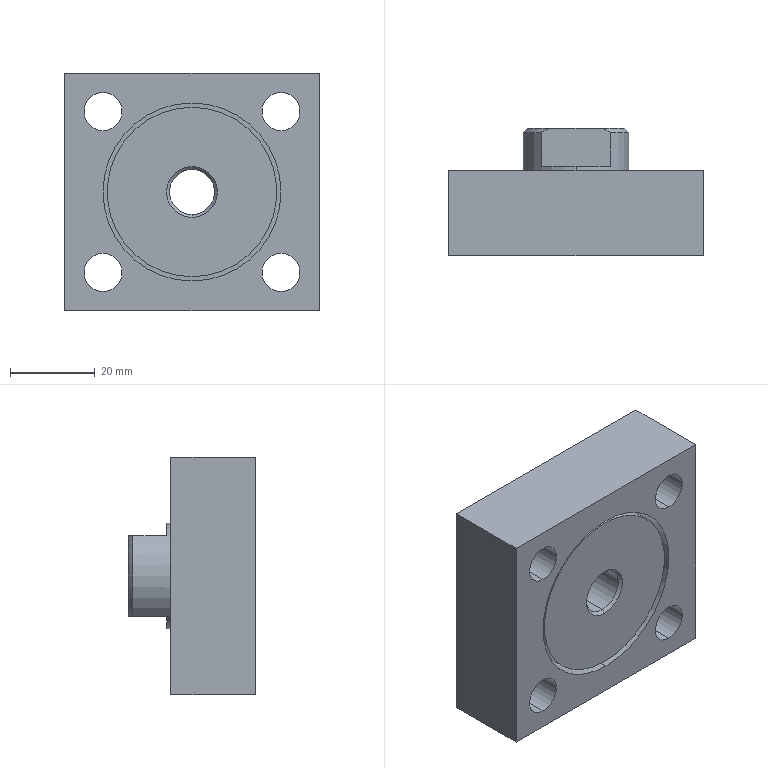Part | SolidWorks | features BaseBody 1 | 1 solid | 51 faces | box 60 x 30 x 56 mm | volume 57044 mm3 | cylinder 26 | plane 18 | cone 7 | commonest cylinder face diameters 9 x8 15 x8 10.647 x2 25 x2 27 x2 40 x2
STEP:
#1=CARTESIAN_POINT('',(21.,11.,11.5));
#2=VERTEX_POINT('',#1);
#3=CARTESIAN_POINT('',(21.,11.,26.5));
#4=VERTEX_POINT('',#3);
#5=CARTESIAN_POINT('',(21.,11.,19.));
#6=DIRECTION('',(0.,1.,0.));
#7=DIRECTION('',(0.,0.,1.));
#8=AXIS2_PLACEMENT_3D('',#5,#6,#7);
#9=CIRCLE('',#8,7.5);
#10=EDGE_CURVE('',#2,#4,#9,.T.);
#11=ORIENTED_EDGE('',*,*,#10,.F.);
#12=CARTESIAN_POINT('',(21.,20.,11.5));
#13=VERTEX_POINT('',#12);
#14=CARTESIAN_POINT('',(21.,0.,11.5));
#15=DIRECTION('',(0.,1.,0.));
#16=VECTOR('',#15,1000.);
#17=LINE('',#14,#16);
#18=EDGE_CURVE('',#2,#13,#17,.T.);
#19=ORIENTED_EDGE('',*,*,#18,.T.);
#20=CARTESIAN_POINT('',(21.,20.,26.5));
#21=VERTEX_POINT('',#20);
#22=CARTESIAN_POINT('',(21.,20.,19.));
#23=DIRECTION('',(0.,-1.,0.));
#24=DIRECTION('',(0.,0.,1.));
#25=AXIS2_PLACEMENT_3D('',#22,#23,#24);
#26=CIRCLE('',#25,7.5);
#27=EDGE_CURVE('',#21,#13,#26,.T.);
#28=ORIENTED_EDGE('',*,*,#27,.F.);
#29=CARTESIAN_POINT('',(21.,0.,26.5));
#30=DIRECTION('',(0.,1.,0.));
#31=VECTOR('',#30,1000.);
#32=LINE('',#29,#31);
#33=EDGE_CURVE('',#4,#21,#32,.T.);
#34=ORIENTED_EDGE('',*,*,#33,.F.);
#35=EDGE_LOOP('',(#11,#19,#28,#34));
#36=FACE_OUTER_BOUND('',#35,.T.);
#37=CARTESIAN_POINT('',(21.,0.,19.));
#38=DIRECTION('',(0.,1.,0.));
#39=DIRECTION('',(0.,0.,1.));
#40=AXIS2_PLACEMENT_3D('',#37,#38,#39);
#41=CYLINDRICAL_SURFACE('',#40,7.5);
#42=ADVANCED_FACE('',(#36),#41,.F.);
#43=CARTESIAN_POINT('',(-21.,11.,11.5));
#44=VERTEX_POINT('',#43);
#45=CARTESIAN_POINT('',(-21.,11.,26.5));
#46=VERTEX_POINT('',#45);
#47=CARTESIAN_POINT('',(-21.,11.,19.));
#48=DIRECTION('',(0.,1.,0.));
#49=DIRECTION('',(0.,0.,1.));
#50=AXIS2_PLACEMENT_3D('',#47,#48,#49);
#51=CIRCLE('',#50,7.5);
#52=EDGE_CURVE('',#44,#46,#51,.T.);
#53=ORIENTED_EDGE('',*,*,#52,.F.);
#54=CARTESIAN_POINT('',(-21.,20.,11.5));
#55=VERTEX_POINT('',#54);
#56=CARTESIAN_POINT('',(-21.,0.,11.5));
#57=DIRECTION('',(0.,1.,0.));
#58=VECTOR('',#57,1000.);
#59=LINE('',#56,#58);
#60=EDGE_CURVE('',#44,#55,#59,.T.);
#61=ORIENTED_EDGE('',*,*,#60,.T.);
#62=CARTESIAN_POINT('',(-21.,20.,26.5));
#63=VERTEX_POINT('',#62);
#64=CARTESIAN_POINT('',(-21.,20.,19.));
#65=DIRECTION('',(0.,-1.,0.));
#66=DIRECTION('',(0.,0.,1.));
#67=AXIS2_PLACEMENT_3D('',#64,#65,#66);
#68=CIRCLE('',#67,7.5);
#69=EDGE_CURVE('',#63,#55,#68,.T.);
#70=ORIENTED_EDGE('',*,*,#69,.F.);
#71=CARTESIAN_POINT('',(-21.,0.,26.5));
#72=DIRECTION('',(0.,1.,0.));
#73=VECTOR('',#72,1000.);
#74=LINE('',#71,#73);
#75=EDGE_CURVE('',#46,#63,#74,.T.);
#76=ORIENTED_EDGE('',*,*,#75,.F.);
#77=EDGE_LOOP('',(#53,#61,#70,#76));
#78=FACE_OUTER_BOUND('',#77,.T.);
#79=CARTESIAN_POINT('',(-21.,0.,19.));
#80=DIRECTION('',(0.,1.,0.));
#81=DIRECTION('',(0.,0.,1.));
#82=AXIS2_PLACEMENT_3D('',#79,#80,#81);
#83=CYLINDRICAL_SURFACE('',#82,7.5);
#84=ADVANCED_FACE('',(#78),#83,.F.);
#85=CARTESIAN_POINT('',(-21.,11.,-26.5));
#86=VERTEX_POINT('',#85);
#87=CARTESIAN_POINT('',(-21.,11.,-11.5));
#88=VERTEX_POINT('',#87);
#89=CARTESIAN_POINT('',(-21.,11.,-19.));
#90=DIRECTION('',(0.,1.,0.));
#91=DIRECTION('',(0.,0.,1.));
#92=AXIS2_PLACEMENT_3D('',#89,#90,#91);
#93=CIRCLE('',#92,7.5);
#94=EDGE_CURVE('',#86,#88,#93,.T.);
#95=ORIENTED_EDGE('',*,*,#94,.F.);
#96=CARTESIAN_POINT('',(-21.,20.,-26.5));
#97=VERTEX_POINT('',#96);
#98=CARTESIAN_POINT('',(-21.,0.,-26.5));
#99=DIRECTION('',(0.,1.,0.));
#100=VECTOR('',#99,1000.);
#101=LINE('',#98,#100);
#102=EDGE_CURVE('',#86,#97,#101,.T.);
#103=ORIENTED_EDGE('',*,*,#102,.T.);
#104=CARTESIAN_POINT('',(-21.,20.,-11.5));
#105=VERTEX_POINT('',#104);
#106=CARTESIAN_POINT('',(-21.,20.,-19.));
#107=DIRECTION('',(0.,-1.,0.));
#108=DIRECTION('',(0.,0.,1.));
#109=AXIS2_PLACEMENT_3D('',#106,#107,#108);
#110=CIRCLE('',#109,7.5);
#111=EDGE_CURVE('',#105,#97,#110,.T.);
#112=ORIENTED_EDGE('',*,*,#111,.F.);
#113=CARTESIAN_POINT('',(-21.,0.,-11.5));
#114=DIRECTION('',(0.,1.,0.));
#115=VECTOR('',#114,1000.);
#116=LINE('',#113,#115);
#117=EDGE_CURVE('',#88,#105,#116,.T.);
#118=ORIENTED_EDGE('',*,*,#117,.F.);
#119=EDGE_LOOP('',(#95,#103,#112,#118));
#120=FACE_OUTER_BOUND('',#119,.T.);
#121=CARTESIAN_POINT('',(-21.,0.,-19.));
#122=DIRECTION('',(0.,1.,0.));
#123=DIRECTION('',(0.,0.,1.));
#124=AXIS2_PLACEMENT_3D('',#121,#122,#123);
#125=CYLINDRICAL_SURFACE('',#124,7.5);
#126=ADVANCED_FACE('',(#120),#125,.F.);
#127=CARTESIAN_POINT('',(21.,11.,-26.5));
#128=VERTEX_POINT('',#127);
#129=CARTESIAN_POINT('',(21.,11.,-11.5));
#130=VERTEX_POINT('',#129);
#131=CARTESIAN_POINT('',(21.,11.,-19.));
#132=DIRECTION('',(0.,1.,0.));
#133=DIRECTION('',(0.,0.,1.));
#134=AXIS2_PLACEMENT_3D('',#131,#132,#133);
#135=CIRCLE('',#134,7.5);
#136=EDGE_CURVE('',#128,#130,#135,.T.);
#137=ORIENTED_EDGE('',*,*,#136,.F.);
#138=CARTESIAN_POINT('',(21.,20.,-26.5));
#139=VERTEX_POINT('',#138);
#140=CARTESIAN_POINT('',(21.,0.,-26.5));
#141=DIRECTION('',(0.,1.,0.));
#142=VECTOR('',#141,1000.);
#143=LINE('',#140,#142);
#144=EDGE_CURVE('',#128,#139,#143,.T.);
#145=ORIENTED_EDGE('',*,*,#144,.T.);
#146=CARTESIAN_POINT('',(21.,20.,-11.5));
#147=VERTEX_POINT('',#146);
#148=CARTESIAN_POINT('',(21.,20.,-19.));
#149=DIRECTION('',(0.,-1.,0.));
#150=DIRECTION('',(0.,0.,1.));
#151=AXIS2_PLACEMENT_3D('',#148,#149,#150);
#152=CIRCLE('',#151,7.5);
#153=EDGE_CURVE('',#147,#139,#152,.T.);
#154=ORIENTED_EDGE('',*,*,#153,.F.);
#155=CARTESIAN_POINT('',(21.,0.,-11.5));
#156=DIRECTION('',(0.,1.,0.));
#157=VECTOR('',#156,1000.);
#158=LINE('',#155,#157);
#159=EDGE_CURVE('',#130,#147,#158,.T.);
#160=ORIENTED_EDGE('',*,*,#159,.F.);
#161=EDGE_LOOP('',(#137,#145,#154,#160));
#162=FACE_OUTER_BOUND('',#161,.T.);
#163=CARTESIAN_POINT('',(21.,0.,-19.));
#164=DIRECTION('',(0.,1.,0.));
#165=DIRECTION('',(0.,0.,1.));
#166=AXIS2_PLACEMENT_3D('',#163,#164,#165);
#167=CYLINDRICAL_SURFACE('',#166,7.5);
#168=ADVANCED_FACE('',(#162),#167,.F.);
#169=CARTESIAN_POINT('',(0.,8.,-13.5));
#170=VERTEX_POINT('',#169);
#171=CARTESIAN_POINT('',(0.,8.,13.5));
#172=VERTEX_POINT('',#171);
#173=CARTESIAN_POINT('',(0.,8.,0.));
#174=DIRECTION('',(0.,1.,0.));
#175=DIRECTION('',(0.,0.,1.));
#176=AXIS2_PLACEMENT_3D('',#173,#174,#175);
#177=CIRCLE('',#176,13.5);
#178=EDGE_CURVE('',#170,#172,#177,.T.);
#179=ORIENTED_EDGE('',*,*,#178,.F.);
#180=CARTESIAN_POINT('',(0.,20.,-13.5));
#181=VERTEX_POINT('',#180);
#182=CARTESIAN_POINT('',(0.,0.,-13.5));
#183=DIRECTION('',(0.,1.,0.));
#184=VECTOR('',#183,1000.);
#185=LINE('',#182,#184);
#186=EDGE_CURVE('',#170,#181,#185,.T.);
#187=ORIENTED_EDGE('',*,*,#186,.T.);
#188=CARTESIAN_POINT('',(0.,20.,13.5));
#189=VERTEX_POINT('',#188);
#190=CARTESIAN_POINT('',(0.,20.,0.));
#191=DIRECTION('',(0.,-1.,0.));
#192=DIRECTION('',(0.,0.,1.));
#193=AXIS2_PLACEMENT_3D('',#190,#191,#192);
#194=CIRCLE('',#193,13.5);
#195=EDGE_CURVE('',#189,#181,#194,.T.);
#196=ORIENTED_EDGE('',*,*,#195,.F.);
#197=CARTESIAN_POINT('',(0.,0.,13.5));
#198=DIRECTION('',(0.,1.,0.));
#199=VECTOR('',#198,1000.);
#200=LINE('',#197,#199);
#201=EDGE_CURVE('',#172,#189,#200,.T.);
#202=ORIENTED_EDGE('',*,*,#201,.F.);
#203=EDGE_LOOP('',(#179,#187,#196,#202));
#204=FACE_OUTER_BOUND('',#203,.T.);
#205=CARTESIAN_POINT('',(0.,0.,0.));
#206=DIRECTION('',(0.,1.,0.));
#207=DIRECTION('',(0.,0.,1.));
#208=AXIS2_PLACEMENT_3D('',#205,#206,#207);
#209=CYLINDRICAL_SURFACE('',#208,13.5);
#210=ADVANCED_FACE('',(#204),#209,.F.);
#211=CARTESIAN_POINT('',(21.,0.,23.5));
#212=VERTEX_POINT('',#211);
#213=CARTESIAN_POINT('',(21.,0.,14.5));
#214=VERTEX_POINT('',#213);
#215=CARTESIAN_POINT('',(21.,0.,19.));
#216=DIRECTION('',(0.,-1.,0.));
#217=DIRECTION('',(0.,0.,1.));
#218=AXIS2_PLACEMENT_3D('',#215,#216,#217);
#219=CIRCLE('',#218,4.5);
#220=EDGE_CURVE('',#212,#214,#219,.T.);
#221=ORIENTED_EDGE('',*,*,#220,.T.);
#222=CARTESIAN_POINT('',(21.,11.,14.5));
#223=VERTEX_POINT('',#222);
#224=CARTESIAN_POINT('',(21.,0.,14.5));
#225=DIRECTION('',(0.,1.,0.));
#226=VECTOR('',#225,1000.);
#227=LINE('',#224,#226);
#228=EDGE_CURVE('',#214,#223,#227,.T.);
#229=ORIENTED_EDGE('',*,*,#228,.T.);
#230=CARTESIAN_POINT('',(21.,11.,23.5));
#231=VERTEX_POINT('',#230);
#232=CARTESIAN_POINT('',(21.,11.,19.));
#233=DIRECTION('',(0.,-1.,0.));
#234=DIRECTION('',(0.,0.,1.));
#235=AXIS2_PLACEMENT_3D('',#232,#233,#234);
#236=CIRCLE('',#235,4.5);
#237=EDGE_CURVE('',#231,#223,#236,.T.);
#238=ORIENTED_EDGE('',*,*,#237,.F.);
#239=CARTESIAN_POINT('',(21.,0.,23.5));
#240=DIRECTION('',(0.,1.,0.));
#241=VECTOR('',#240,1000.);
#242=LINE('',#239,#241);
#243=EDGE_CURVE('',#212,#231,#242,.T.);
#244=ORIENTED_EDGE('',*,*,#243,.F.);
#245=EDGE_LOOP('',(#221,#229,#238,#244));
#246=FACE_OUTER_BOUND('',#245,.T.);
#247=CARTESIAN_POINT('',(21.,0.,19.));
#248=DIRECTION('',(0.,1.,0.));
#249=DIRECTION('',(0.,0.,1.));
#250=AXIS2_PLACEMENT_3D('',#247,#248,#249);
#251=CYLINDRICAL_SURFACE('',#250,4.5);
#252=ADVANCED_FACE('',(#246),#251,.F.);
#253=CARTESIAN_POINT('',(-21.,0.,23.5));
#254=VERTEX_POINT('',#253);
#255=CARTESIAN_POINT('',(-21.,0.,14.5));
#256=VERTEX_POINT('',#255);
#257=CARTESIAN_POINT('',(-21.,0.,19.));
#258=DIRECTION('',(0.,-1.,0.));
#259=DIRECTION('',(0.,0.,1.));
#260=AXIS2_PLACEMENT_3D('',#257,#258,#259);
#261=CIRCLE('',#260,4.5);
#262=EDGE_CURVE('',#254,#256,#261,.T.);
#263=ORIENTED_EDGE('',*,*,#262,.T.);
#264=CARTESIAN_POINT('',(-21.,11.,14.5));
#265=VERTEX_POINT('',#264);
#266=CARTESIAN_POINT('',(-21.,0.,14.5));
#267=DIRECTION('',(0.,1.,0.));
#268=VECTOR('',#267,1000.);
#269=LINE('',#266,#268);
#270=EDGE_CURVE('',#256,#265,#269,.T.);
#271=ORIENTED_EDGE('',*,*,#270,.T.);
#272=CARTESIAN_POINT('',(-21.,11.,23.5));
#273=VERTEX_POINT('',#272);
#274=CARTESIAN_POINT('',(-21.,11.,19.));
#275=DIRECTION('',(0.,-1.,0.));
#276=DIRECTION('',(0.,0.,1.));
#277=AXIS2_PLACEMENT_3D('',#274,#275,#276);
#278=CIRCLE('',#277,4.5);
#279=EDGE_CURVE('',#273,#265,#278,.T.);
#280=ORIENTED_EDGE('',*,*,#279,.F.);
#281=CARTESIAN_POINT('',(-21.,0.,23.5));
#282=DIRECTION('',(0.,1.,0.));
#283=VECTOR('',#282,1000.);
#284=LINE('',#281,#283);
#285=EDGE_CURVE('',#254,#273,#284,.T.);
#286=ORIENTED_EDGE('',*,*,#285,.F.);
#287=EDGE_LOOP('',(#263,#271,#280,#286));
#288=FACE_OUTER_BOUND('',#287,.T.);
#289=CARTESIAN_POINT('',(-21.,0.,19.));
#290=DIRECTION('',(0.,1.,0.));
#291=DIRECTION('',(0.,0.,1.));
#292=AXIS2_PLACEMENT_3D('',#289,#290,#291);
#293=CYLINDRICAL_SURFACE('',#292,4.5);
#294=ADVANCED_FACE('',(#288),#293,.F.);
#295=CARTESIAN_POINT('',(-21.,0.,-14.5));
#296=VERTEX_POINT('',#295);
#297=CARTESIAN_POINT('',(-21.,0.,-23.5));
#298=VERTEX_POINT('',#297);
#299=CARTESIAN_POINT('',(-21.,0.,-19.));
#300=DIRECTION('',(0.,-1.,0.));
#301=DIRECTION('',(0.,0.,1.));
#302=AXIS2_PLACEMENT_3D('',#299,#300,#301);
#303=CIRCLE('',#302,4.5);
#304=EDGE_CURVE('',#296,#298,#303,.T.);
#305=ORIENTED_EDGE('',*,*,#304,.T.);
#306=CARTESIAN_POINT('',(-21.,11.,-23.5));
#307=VERTEX_POINT('',#306);
#308=CARTESIAN_POINT('',(-21.,0.,-23.5));
#309=DIRECTION('',(0.,1.,0.));
#310=VECTOR('',#309,1000.);
#311=LINE('',#308,#310);
#312=EDGE_CURVE('',#298,#307,#311,.T.);
#313=ORIENTED_EDGE('',*,*,#312,.T.);
#314=CARTESIAN_POINT('',(-21.,11.,-14.5));
#315=VERTEX_POINT('',#314);
#316=CARTESIAN_POINT('',(-21.,11.,-19.));
#317=DIRECTION('',(0.,-1.,0.));
#318=DIRECTION('',(0.,0.,1.));
#319=AXIS2_PLACEMENT_3D('',#316,#317,#318);
#320=CIRCLE('',#319,4.5);
#321=EDGE_CURVE('',#315,#307,#320,.T.);
#322=ORIENTED_EDGE('',*,*,#321,.F.);
#323=CARTESIAN_POINT('',(-21.,0.,-14.5));
#324=DIRECTION('',(0.,1.,0.));
#325=VECTOR('',#324,1000.);
#326=LINE('',#323,#325);
#327=EDGE_CURVE('',#296,#315,#326,.T.);
#328=ORIENTED_EDGE('',*,*,#327,.F.);
#329=EDGE_LOOP('',(#305,#313,#322,#328));
#330=FACE_OUTER_BOUND('',#329,.T.);
#331=CARTESIAN_POINT('',(-21.,0.,-19.));
#332=DIRECTION('',(0.,1.,0.));
#333=DIRECTION('',(0.,0.,1.));
#334=AXIS2_PLACEMENT_3D('',#331,#332,#333);
#335=CYLINDRICAL_SURFACE('',#334,4.5);
#336=ADVANCED_FACE('',(#330),#335,.F.);
#337=CARTESIAN_POINT('',(21.,0.,-14.5));
#338=VERTEX_POINT('',#337);
#339=CARTESIAN_POINT('',(21.,0.,-23.5));
#340=VERTEX_POINT('',#339);
#341=CARTESIAN_POINT('',(21.,0.,-19.));
#342=DIRECTION('',(0.,-1.,0.));
#343=DIRECTION('',(0.,0.,1.));
#344=AXIS2_PLACEMENT_3D('',#341,#342,#343);
#345=CIRCLE('',#344,4.5);
#346=EDGE_CURVE('',#338,#340,#345,.T.);
#347=ORIENTED_EDGE('',*,*,#346,.T.);
#348=CARTESIAN_POINT('',(21.,11.,-23.5));
#349=VERTEX_POINT('',#348);
#350=CARTESIAN_POINT('',(21.,0.,-23.5));
#351=DIRECTION('',(0.,1.,0.));
#352=VECTOR('',#351,1000.);
#353=LINE('',#350,#352);
#354=EDGE_CURVE('',#340,#349,#353,.T.);
#355=ORIENTED_EDGE('',*,*,#354,.T.);
#356=CARTESIAN_POINT('',(21.,11.,-14.5));
#357=VERTEX_POINT('',#356);
#358=CARTESIAN_POINT('',(21.,11.,-19.));
#359=DIRECTION('',(0.,-1.,0.));
#360=DIRECTION('',(0.,0.,1.));
#361=AXIS2_PLACEMENT_3D('',#358,#359,#360);
#362=CIRCLE('',#361,4.5);
#363=EDGE_CURVE('',#357,#349,#362,.T.);
#364=ORIENTED_EDGE('',*,*,#363,.F.);
#365=CARTESIAN_POINT('',(21.,0.,-14.5));
#366=DIRECTION('',(0.,1.,0.));
#367=VECTOR('',#366,1000.);
#368=LINE('',#365,#367);
#369=EDGE_CURVE('',#338,#357,#368,.T.);
#370=ORIENTED_EDGE('',*,*,#369,.F.);
#371=EDGE_LOOP('',(#347,#355,#364,#370));
#372=FACE_OUTER_BOUND('',#371,.T.);
#373=CARTESIAN_POINT('',(21.,0.,-19.));
#374=DIRECTION('',(0.,1.,0.));
#375=DIRECTION('',(0.,0.,1.));
#376=AXIS2_PLACEMENT_3D('',#373,#374,#375);
#377=CYLINDRICAL_SURFACE('',#376,4.5);
#378=ADVANCED_FACE('',(#372),#377,.F.);
#379=CARTESIAN_POINT('',(0.,0.,21.));
#380=VERTEX_POINT('',#379);
#381=CARTESIAN_POINT('',(0.,0.,-21.));
#382=VERTEX_POINT('',#381);
#383=CARTESIAN_POINT('',(0.,0.,0.));
#384=DIRECTION('',(0.,-1.,0.));
#385=DIRECTION('',(0.,0.,1.));
#386=AXIS2_PLACEMENT_3D('',#383,#384,#385);
#387=CIRCLE('',#386,21.);
#388=EDGE_CURVE('',#380,#382,#387,.T.);
#389=ORIENTED_EDGE('',*,*,#388,.T.);
#390=CARTESIAN_POINT('',(0.,8.,-21.));
#391=VERTEX_POINT('',#390);
#392=CARTESIAN_POINT('',(0.,0.,-21.));
#393=DIRECTION('',(0.,1.,0.));
#394=VECTOR('',#393,1000.);
#395=LINE('',#392,#394);
#396=EDGE_CURVE('',#382,#391,#395,.T.);
#397=ORIENTED_EDGE('',*,*,#396,.T.);
#398=CARTESIAN_POINT('',(0.,8.,21.));
#399=VERTEX_POINT('',#398);
#400=CARTESIAN_POINT('',(0.,8.,0.));
#401=DIRECTION('',(0.,-1.,0.));
#402=DIRECTION('',(0.,0.,1.));
#403=AXIS2_PLACEMENT_3D('',#400,#401,#402);
#404=CIRCLE('',#403,21.);
#405=EDGE_CURVE('',#399,#391,#404,.T.);
#406=ORIENTED_EDGE('',*,*,#405,.F.);
#407=CARTESIAN_POINT('',(0.,0.,21.));
#408=DIRECTION('',(0.,1.,0.));
#409=VECTOR('',#408,1000.);
#410=LINE('',#407,#409);
#411=EDGE_CURVE('',#380,#399,#410,.T.);
#412=ORIENTED_EDGE('',*,*,#411,.F.);
#413=EDGE_LOOP('',(#389,#397,#406,#412));
#414=FACE_OUTER_BOUND('',#413,.T.);
#415=CARTESIAN_POINT('',(0.,0.,0.));
#416=DIRECTION('',(0.,1.,0.));
#417=DIRECTION('',(0.,0.,1.));
#418=AXIS2_PLACEMENT_3D('',#415,#416,#417);
#419=CYLINDRICAL_SURFACE('',#418,21.);
#420=ADVANCED_FACE('',(#414),#419,.F.);
#421=CARTESIAN_POINT('',(0.,8.,-12.5));
#422=VERTEX_POINT('',#421);
#423=CARTESIAN_POINT('',(0.,8.,12.5));
#424=VERTEX_POINT('',#423);
#425=CARTESIAN_POINT('',(0.,8.,0.));
#426=DIRECTION('',(0.,-1.,0.));
#427=DIRECTION('',(0.,0.,1.));
#428=AXIS2_PLACEMENT_3D('',#425,#426,#427);
#429=CIRCLE('',#428,12.5);
#430=EDGE_CURVE('',#422,#424,#429,.T.);
#431=ORIENTED_EDGE('',*,*,#430,.F.);
#432=CARTESIAN_POINT('',(0.,21.,-12.5));
#433=VERTEX_POINT('',#432);
#434=CARTESIAN_POINT('',(0.,0.5,-12.5));
#435=DIRECTION('',(0.,1.,0.));
#436=VECTOR('',#435,1000.);
#437=LINE('',#434,#436);
#438=EDGE_CURVE('',#422,#433,#437,.T.);
#439=ORIENTED_EDGE('',*,*,#438,.T.);
#440=CARTESIAN_POINT('',(8.124,21.,-9.5));
#441=VERTEX_POINT('',#440);
#442=CARTESIAN_POINT('',(0.,21.,0.));
#443=DIRECTION('',(0.,-1.,0.));
#444=DIRECTION('',(0.,0.,1.));
#445=AXIS2_PLACEMENT_3D('',#442,#443,#444);
#446=CIRCLE('',#445,12.5);
#447=EDGE_CURVE('',#433,#441,#446,.T.);
#448=ORIENTED_EDGE('',*,*,#447,.T.);
#449=CARTESIAN_POINT('',(8.124,29.,-9.5));
#450=VERTEX_POINT('',#449);
#451=CARTESIAN_POINT('',(8.124,0.5,-9.5));
#452=DIRECTION('',(0.,1.,0.));
#453=VECTOR('',#452,1000.);
#454=LINE('',#451,#453);
#455=EDGE_CURVE('',#441,#450,#454,.T.);
#456=ORIENTED_EDGE('',*,*,#455,.T.);
#457=CARTESIAN_POINT('',(12.5,29.,0.));
#458=VERTEX_POINT('',#457);
#459=CARTESIAN_POINT('',(0.,29.,0.));
#460=DIRECTION('',(0.,-1.,0.));
#461=DIRECTION('',(0.,0.,1.));
#462=AXIS2_PLACEMENT_3D('',#459,#460,#461);
#463=CIRCLE('',#462,12.5);
#464=EDGE_CURVE('',#450,#458,#463,.T.);
#465=ORIENTED_EDGE('',*,*,#464,.T.);
#466=CARTESIAN_POINT('',(8.124,29.,9.5));
#467=VERTEX_POINT('',#466);
#468=CARTESIAN_POINT('',(0.,29.,0.));
#469=DIRECTION('',(0.,-1.,0.));
#470=DIRECTION('',(0.,0.,1.));
#471=AXIS2_PLACEMENT_3D('',#468,#469,#470);
#472=CIRCLE('',#471,12.5);
#473=EDGE_CURVE('',#458,#467,#472,.T.);
#474=ORIENTED_EDGE('',*,*,#473,.T.);
#475=CARTESIAN_POINT('',(8.124,21.,9.5));
#476=VERTEX_POINT('',#475);
#477=CARTESIAN_POINT('',(8.124,0.5,9.5));
#478=DIRECTION('',(0.,-1.,0.));
#479=VECTOR('',#478,1000.);
#480=LINE('',#477,#479);
#481=EDGE_CURVE('',#467,#476,#480,.T.);
#482=ORIENTED_EDGE('',*,*,#481,.T.);
#483=CARTESIAN_POINT('',(0.,21.,12.5));
#484=VERTEX_POINT('',#483);
#485=CARTESIAN_POINT('',(0.,21.,0.));
#486=DIRECTION('',(0.,-1.,0.));
#487=DIRECTION('',(0.,0.,1.));
#488=AXIS2_PLACEMENT_3D('',#485,#486,#487);
#489=CIRCLE('',#488,12.5);
#490=EDGE_CURVE('',#476,#484,#489,.T.);
#491=ORIENTED_EDGE('',*,*,#490,.T.);
#492=CARTESIAN_POINT('',(0.,0.5,12.5));
#493=DIRECTION('',(0.,1.,0.));
#494=VECTOR('',#493,1000.);
#495=LINE('',#492,#494);
#496=EDGE_CURVE('',#424,#484,#495,.T.);
#497=ORIENTED_EDGE('',*,*,#496,.F.);
#498=EDGE_LOOP('',(#431,#439,#448,#456,#465,#474,#482,#491,#497));
#499=FACE_OUTER_BOUND('',#498,.T.);
#500=CARTESIAN_POINT('',(0.,0.5,0.));
#501=DIRECTION('',(0.,1.,0.));
#502=DIRECTION('',(0.,0.,1.));
#503=AXIS2_PLACEMENT_3D('',#500,#501,#502);
#504=CYLINDRICAL_SURFACE('',#503,12.5);
#505=ADVANCED_FACE('',(#499),#504,.T.);
#506=CARTESIAN_POINT('',(6.481,30.,-9.5));
#507=VERTEX_POINT('',#506);
#508=CARTESIAN_POINT('',(11.5,30.,0.));
#509=VERTEX_POINT('',#508);
#510=CARTESIAN_POINT('',(0.,30.,0.));
#511=DIRECTION('',(0.,-1.,0.));
#512=DIRECTION('',(1.,0.,0.));
#513=AXIS2_PLACEMENT_3D('',#510,#511,#512);
#514=CIRCLE('',#513,11.5);
#515=EDGE_CURVE('',#507,#509,#514,.T.);
#516=ORIENTED_EDGE('',*,*,#515,.T.);
#517=CARTESIAN_POINT('',(12.5,29.,0.));
#518=DIRECTION('',(0.7071,-0.7071,0.));
#519=VECTOR('',#518,1000.);
#520=LINE('',#517,#519);
#521=EDGE_CURVE('',#509,#458,#520,.T.);
#522=ORIENTED_EDGE('',*,*,#521,.T.);
#523=ORIENTED_EDGE('',*,*,#464,.F.);
#524=CARTESIAN_POINT('',(8.124,29.,-9.5));
#525=CARTESIAN_POINT('',(7.586,29.35,-9.5));
#526=CARTESIAN_POINT('',(7.04,29.685,-9.5));
#527=CARTESIAN_POINT('',(6.481,30.,-9.5));
#528=B_SPLINE_CURVE_WITH_KNOTS('',3,(#524,#525,#526,#527),.UNSPECIFIED.,.F.,.F.,(4,4),(0.,0.001924),.UNSPECIFIED.);
#529=EDGE_CURVE('',#450,#507,#528,.T.);
#530=ORIENTED_EDGE('',*,*,#529,.T.);
#531=EDGE_LOOP('',(#516,#522,#523,#530));
#532=FACE_OUTER_BOUND('',#531,.T.);
#533=CARTESIAN_POINT('',(0.,29.,0.));
#534=DIRECTION('',(0.,-1.,0.));
#535=DIRECTION('',(1.,0.,0.));
#536=AXIS2_PLACEMENT_3D('',#533,#534,#535);
#537=CONICAL_SURFACE('',#536,12.5,0.7854);
#538=ADVANCED_FACE('',(#532),#537,.T.);
#539=CARTESIAN_POINT('',(0.,0.5,20.));
#540=VERTEX_POINT('',#539);
#541=CARTESIAN_POINT('',(0.,0.5,-20.));
#542=VERTEX_POINT('',#541);
#543=CARTESIAN_POINT('',(0.,0.5,0.));
#544=DIRECTION('',(0.,1.,0.));
#545=DIRECTION('',(0.,0.,1.));
#546=AXIS2_PLACEMENT_3D('',#543,#544,#545);
#547=CIRCLE('',#546,20.);
#548=EDGE_CURVE('',#540,#542,#547,.T.);
#549=ORIENTED_EDGE('',*,*,#548,.T.);
#550=CARTESIAN_POINT('',(0.,8.,-20.));
#551=VERTEX_POINT('',#550);
#552=CARTESIAN_POINT('',(0.,0.5,-20.));
#553=DIRECTION('',(0.,1.,0.));
#554=VECTOR('',#553,1000.);
#555=LINE('',#552,#554);
#556=EDGE_CURVE('',#542,#551,#555,.T.);
#557=ORIENTED_EDGE('',*,*,#556,.T.);
#558=CARTESIAN_POINT('',(0.,8.,20.));
#559=VERTEX_POINT('',#558);
#560=CARTESIAN_POINT('',(0.,8.,0.));
#561=DIRECTION('',(0.,1.,0.));
#562=DIRECTION('',(0.,0.,1.));
#563=AXIS2_PLACEMENT_3D('',#560,#561,#562);
#564=CIRCLE('',#563,20.);
#565=EDGE_CURVE('',#559,#551,#564,.T.);
#566=ORIENTED_EDGE('',*,*,#565,.F.);
#567=CARTESIAN_POINT('',(0.,0.5,20.));
#568=DIRECTION('',(0.,1.,0.));
#569=VECTOR('',#568,1000.);
#570=LINE('',#567,#569);
#571=EDGE_CURVE('',#540,#559,#570,.T.);
#572=ORIENTED_EDGE('',*,*,#571,.F.);
#573=EDGE_LOOP('',(#549,#557,#566,#572));
#574=FACE_OUTER_BOUND('',#573,.T.);
#575=CARTESIAN_POINT('',(0.,0.5,0.));
#576=DIRECTION('',(0.,1.,0.));
#577=DIRECTION('',(0.,0.,1.));
#578=AXIS2_PLACEMENT_3D('',#575,#576,#577);
#579=CYLINDRICAL_SURFACE('',#578,20.);
#580=ADVANCED_FACE('',(#574),#579,.T.);
#581=CARTESIAN_POINT('',(0.,29.324,-5.323));
#582=VERTEX_POINT('',#581);
#583=CARTESIAN_POINT('',(0.,29.324,5.323));
#584=VERTEX_POINT('',#583);
#585=CARTESIAN_POINT('',(0.,29.324,0.));
#586=DIRECTION('',(0.,1.,0.));
#587=DIRECTION('',(0.,0.,1.));
#588=AXIS2_PLACEMENT_3D('',#585,#586,#587);
#589=CIRCLE('',#588,5.323);
#590=EDGE_CURVE('',#582,#584,#589,.T.);
#591=ORIENTED_EDGE('',*,*,#590,.F.);
#592=CARTESIAN_POINT('',(0.,30.,-6.));
#593=VERTEX_POINT('',#592);
#594=CARTESIAN_POINT('',(0.,30.,-6.));
#595=DIRECTION('',(0.,0.7071,-0.7071));
#596=VECTOR('',#595,1000.);
#597=LINE('',#594,#596);
#598=EDGE_CURVE('',#582,#593,#597,.T.);
#599=ORIENTED_EDGE('',*,*,#598,.T.);
#600=CARTESIAN_POINT('',(0.,30.,6.));
#601=VERTEX_POINT('',#600);
#602=CARTESIAN_POINT('',(0.,30.,0.));
#603=DIRECTION('',(0.,-1.,0.));
#604=DIRECTION('',(0.,0.,1.));
#605=AXIS2_PLACEMENT_3D('',#602,#603,#604);
#606=CIRCLE('',#605,6.);
#607=EDGE_CURVE('',#601,#593,#606,.T.);
#608=ORIENTED_EDGE('',*,*,#607,.F.);
#609=CARTESIAN_POINT('',(0.,30.,6.));
#610=DIRECTION('',(0.,0.7071,0.7071));
#611=VECTOR('',#610,1000.);
#612=LINE('',#609,#611);
#613=EDGE_CURVE('',#584,#601,#612,.T.);
#614=ORIENTED_EDGE('',*,*,#613,.F.);
#615=EDGE_LOOP('',(#591,#599,#608,#614));
#616=FACE_OUTER_BOUND('',#615,.T.);
#617=CARTESIAN_POINT('',(0.,30.,0.));
#618=DIRECTION('',(0.,1.,0.));
#619=DIRECTION('',(0.,0.,1.));
#620=AXIS2_PLACEMENT_3D('',#617,#618,#619);
#621=CONICAL_SURFACE('',#620,6.,0.7854);
#622=ADVANCED_FACE('',(#616),#621,.F.);
#623=CARTESIAN_POINT('',(0.,1.176,5.324));
#624=VERTEX_POINT('',#623);
#625=CARTESIAN_POINT('',(0.,1.176,-5.324));
#626=VERTEX_POINT('',#625);
#627=CARTESIAN_POINT('',(0.,1.176,0.));
#628=DIRECTION('',(0.,-1.,0.));
#629=DIRECTION('',(0.,0.,-1.));
#630=AXIS2_PLACEMENT_3D('',#627,#628,#629);
#631=CIRCLE('',#630,5.324);
#632=EDGE_CURVE('',#624,#626,#631,.T.);
#633=ORIENTED_EDGE('',*,*,#632,.F.);
#634=CARTESIAN_POINT('',(0.,0.5,6.));
#635=VERTEX_POINT('',#634);
#636=CARTESIAN_POINT('',(0.,0.5,6.));
#637=DIRECTION('',(0.,-0.7071,0.7071));
#638=VECTOR('',#637,1000.);
#639=LINE('',#636,#638);
#640=EDGE_CURVE('',#624,#635,#639,.T.);
#641=ORIENTED_EDGE('',*,*,#640,.T.);
#642=CARTESIAN_POINT('',(0.,0.5,-6.));
#643=VERTEX_POINT('',#642);
#644=CARTESIAN_POINT('',(0.,0.5,0.));
#645=DIRECTION('',(0.,1.,0.));
#646=DIRECTION('',(0.,0.,-1.));
#647=AXIS2_PLACEMENT_3D('',#644,#645,#646);
#648=CIRCLE('',#647,6.);
#649=EDGE_CURVE('',#643,#635,#648,.T.);
#650=ORIENTED_EDGE('',*,*,#649,.F.);
#651=CARTESIAN_POINT('',(0.,0.5,-6.));
#652=DIRECTION('',(0.,-0.7071,-0.7071));
#653=VECTOR('',#652,1000.);
#654=LINE('',#651,#653);
#655=EDGE_CURVE('',#626,#643,#654,.T.);
#656=ORIENTED_EDGE('',*,*,#655,.F.);
#657=EDGE_LOOP('',(#633,#641,#650,#656));
#658=FACE_OUTER_BOUND('',#657,.T.);
#659=CARTESIAN_POINT('',(0.,0.5,0.));
#660=DIRECTION('',(0.,-1.,0.));
#661=DIRECTION('',(0.,0.,-1.));
#662=AXIS2_PLACEMENT_3D('',#659,#660,#661);
#663=CONICAL_SURFACE('',#662,6.,0.7854);
#664=ADVANCED_FACE('',(#658),#663,.F.);
#665=ORIENTED_EDGE('',*,*,#632,.T.);
#666=CARTESIAN_POINT('',(0.,0.5,-5.324));
#667=DIRECTION('',(0.,1.,0.));
#668=VECTOR('',#667,1000.);
#669=LINE('',#666,#668);
#670=EDGE_CURVE('',#626,#582,#669,.T.);
#671=ORIENTED_EDGE('',*,*,#670,.T.);
#672=ORIENTED_EDGE('',*,*,#590,.T.);
#673=CARTESIAN_POINT('',(0.,0.5,5.324));
#674=DIRECTION('',(0.,1.,0.));
#675=VECTOR('',#674,1000.);
#676=LINE('',#673,#675);
#677=EDGE_CURVE('',#624,#584,#676,.T.);
#678=ORIENTED_EDGE('',*,*,#677,.F.);
#679=EDGE_LOOP('',(#665,#671,#672,#678));
#680=FACE_OUTER_BOUND('',#679,.T.);
#681=CARTESIAN_POINT('',(0.,0.5,0.));
#682=DIRECTION('',(0.,1.,0.));
#683=DIRECTION('',(0.,0.,1.));
#684=AXIS2_PLACEMENT_3D('',#681,#682,#683);
#685=CYLINDRICAL_SURFACE('',#684,5.324);
#686=ADVANCED_FACE('',(#680),#685,.F.);
#687=CARTESIAN_POINT('',(30.,20.,28.));
#688=VERTEX_POINT('',#687);
#689=CARTESIAN_POINT('',(30.,20.,-28.));
#690=VERTEX_POINT('',#689);
#691=CARTESIAN_POINT('',(30.,20.,0.));
#692=DIRECTION('',(0.,0.,-1.));
#693=VECTOR('',#692,1000.);
#694=LINE('',#691,#693);
#695=EDGE_CURVE('',#688,#690,#694,.T.);
#696=ORIENTED_EDGE('',*,*,#695,.T.);
#697=CARTESIAN_POINT('',(-30.,20.,-28.));
#698=VERTEX_POINT('',#697);
#699=CARTESIAN_POINT('',(0.,20.,-28.));
#700=DIRECTION('',(-1.,0.,0.));
#701=VECTOR('',#700,1000.);
#702=LINE('',#699,#701);
#703=EDGE_CURVE('',#690,#698,#702,.T.);
#704=ORIENTED_EDGE('',*,*,#703,.T.);
#705=CARTESIAN_POINT('',(-30.,20.,28.));
#706=VERTEX_POINT('',#705);
#707=CARTESIAN_POINT('',(-30.,20.,0.));
#708=DIRECTION('',(0.,0.,1.));
#709=VECTOR('',#708,1000.);
#710=LINE('',#707,#709);
#711=EDGE_CURVE('',#698,#706,#710,.T.);
#712=ORIENTED_EDGE('',*,*,#711,.T.);
#713=CARTESIAN_POINT('',(0.,20.,28.));
#714=DIRECTION('',(1.,0.,0.));
#715=VECTOR('',#714,1000.);
#716=LINE('',#713,#715);
#717=EDGE_CURVE('',#706,#688,#716,.T.);
#718=ORIENTED_EDGE('',*,*,#717,.T.);
#719=EDGE_LOOP('',(#696,#704,#712,#718));
#720=FACE_OUTER_BOUND('',#719,.T.);
#721=ORIENTED_EDGE('',*,*,#27,.T.);
#722=CARTESIAN_POINT('',(21.,20.,19.));
#723=DIRECTION('',(0.,-1.,0.));
#724=DIRECTION('',(0.,0.,1.));
#725=AXIS2_PLACEMENT_3D('',#722,#723,#724);
#726=CIRCLE('',#725,7.5);
#727=EDGE_CURVE('',#13,#21,#726,.T.);
#728=ORIENTED_EDGE('',*,*,#727,.T.);
#729=EDGE_LOOP('',(#721,#728));
#730=FACE_BOUND('',#729,.T.);
#731=ORIENTED_EDGE('',*,*,#69,.T.);
#732=CARTESIAN_POINT('',(-21.,20.,19.));
#733=DIRECTION('',(0.,-1.,0.));
#734=DIRECTION('',(0.,0.,1.));
#735=AXIS2_PLACEMENT_3D('',#732,#733,#734);
#736=CIRCLE('',#735,7.5);
#737=EDGE_CURVE('',#55,#63,#736,.T.);
#738=ORIENTED_EDGE('',*,*,#737,.T.);
#739=EDGE_LOOP('',(#731,#738));
#740=FACE_BOUND('',#739,.T.);
#741=ORIENTED_EDGE('',*,*,#111,.T.);
#742=CARTESIAN_POINT('',(-21.,20.,-19.));
#743=DIRECTION('',(0.,-1.,0.));
#744=DIRECTION('',(0.,0.,1.));
#745=AXIS2_PLACEMENT_3D('',#742,#743,#744);
#746=CIRCLE('',#745,7.5);
#747=EDGE_CURVE('',#97,#105,#746,.T.);
#748=ORIENTED_EDGE('',*,*,#747,.T.);
#749=EDGE_LOOP('',(#741,#748));
#750=FACE_BOUND('',#749,.T.);
#751=ORIENTED_EDGE('',*,*,#153,.T.);
#752=CARTESIAN_POINT('',(21.,20.,-19.));
#753=DIRECTION('',(0.,-1.,0.));
#754=DIRECTION('',(0.,0.,1.));
#755=AXIS2_PLACEMENT_3D('',#752,#753,#754);
#756=CIRCLE('',#755,7.5);
#757=EDGE_CURVE('',#139,#147,#756,.T.);
#758=ORIENTED_EDGE('',*,*,#757,.T.);
#759=EDGE_LOOP('',(#751,#758));
#760=FACE_BOUND('',#759,.T.);
#761=ORIENTED_EDGE('',*,*,#195,.T.);
#762=CARTESIAN_POINT('',(0.,20.,0.));
#763=DIRECTION('',(0.,-1.,0.));
#764=DIRECTION('',(0.,0.,1.));
#765=AXIS2_PLACEMENT_3D('',#762,#763,#764);
#766=CIRCLE('',#765,13.5);
#767=EDGE_CURVE('',#181,#189,#766,.T.);
#768=ORIENTED_EDGE('',*,*,#767,.T.);
#769=EDGE_LOOP('',(#761,#768));
#770=FACE_BOUND('',#769,.T.);
#771=CARTESIAN_POINT('',(0.,20.,0.));
#772=DIRECTION('',(0.,1.,0.));
#773=DIRECTION('',(0.,0.,1.));
#774=AXIS2_PLACEMENT_3D('',#771,#772,#773);
#775=PLANE('',#774);
#776=ADVANCED_FACE('',(#720,#730,#740,#750,#760,#770),#775,.T.);
#777=CARTESIAN_POINT('',(-30.,0.,-28.));
#778=VERTEX_POINT('',#777);
#779=CARTESIAN_POINT('',(-30.,20.,-28.));
#780=DIRECTION('',(0.,-1.,0.));
#781=VECTOR('',#780,1000.);
#782=LINE('',#779,#781);
#783=EDGE_CURVE('',#698,#778,#782,.T.);
#784=ORIENTED_EDGE('',*,*,#783,.F.);
#785=ORIENTED_EDGE('',*,*,#703,.F.);
#786=CARTESIAN_POINT('',(30.,0.,-28.));
#787=VERTEX_POINT('',#786);
#788=CARTESIAN_POINT('',(30.,20.,-28.));
#789=DIRECTION('',(0.,1.,0.));
#790=VECTOR('',#789,1000.);
#791=LINE('',#788,#790);
#792=EDGE_CURVE('',#787,#690,#791,.T.);
#793=ORIENTED_EDGE('',*,*,#792,.F.);
#794=CARTESIAN_POINT('',(30.,0.,-28.));
#795=DIRECTION('',(1.,0.,0.));
#796=VECTOR('',#795,1000.);
#797=LINE('',#794,#796);
#798=EDGE_CURVE('',#778,#787,#797,.T.);
#799=ORIENTED_EDGE('',*,*,#798,.F.);
#800=EDGE_LOOP('',(#784,#785,#793,#799));
#801=FACE_OUTER_BOUND('',#800,.T.);
#802=CARTESIAN_POINT('',(30.,20.,-28.));
#803=DIRECTION('',(0.,0.,1.));
#804=DIRECTION('',(1.,0.,0.));
#805=AXIS2_PLACEMENT_3D('',#802,#803,#804);
#806=PLANE('',#805);
#807=ADVANCED_FACE('',(#801),#806,.F.);
#808=ORIENTED_EDGE('',*,*,#792,.T.);
#809=ORIENTED_EDGE('',*,*,#695,.F.);
#810=CARTESIAN_POINT('',(30.,0.,28.));
#811=VERTEX_POINT('',#810);
#812=CARTESIAN_POINT('',(30.,20.,28.));
#813=DIRECTION('',(0.,1.,0.));
#814=VECTOR('',#813,1000.);
#815=LINE('',#812,#814);
#816=EDGE_CURVE('',#811,#688,#815,.T.);
#817=ORIENTED_EDGE('',*,*,#816,.F.);
#818=CARTESIAN_POINT('',(30.,0.,28.));
#819=DIRECTION('',(0.,0.,1.));
#820=VECTOR('',#819,1000.);
#821=LINE('',#818,#820);
#822=EDGE_CURVE('',#787,#811,#821,.T.);
#823=ORIENTED_EDGE('',*,*,#822,.F.);
#824=EDGE_LOOP('',(#808,#809,#817,#823));
#825=FACE_OUTER_BOUND('',#824,.T.);
#826=CARTESIAN_POINT('',(30.,20.,28.));
#827=DIRECTION('',(-1.,0.,0.));
#828=DIRECTION('',(0.,0.,1.));
#829=AXIS2_PLACEMENT_3D('',#826,#827,#828);
#830=PLANE('',#829);
#831=ADVANCED_FACE('',(#825),#830,.F.);
#832=ORIENTED_EDGE('',*,*,#816,.T.);
#833=ORIENTED_EDGE('',*,*,#717,.F.);
#834=CARTESIAN_POINT('',(-30.,0.,28.));
#835=VERTEX_POINT('',#834);
#836=CARTESIAN_POINT('',(-30.,20.,28.));
#837=DIRECTION('',(0.,1.,0.));
#838=VECTOR('',#837,1000.);
#839=LINE('',#836,#838);
#840=EDGE_CURVE('',#835,#706,#839,.T.);
#841=ORIENTED_EDGE('',*,*,#840,.F.);
#842=CARTESIAN_POINT('',(-30.,0.,28.));
#843=DIRECTION('',(-1.,0.,0.));
#844=VECTOR('',#843,1000.);
#845=LINE('',#842,#844);
#846=EDGE_CURVE('',#811,#835,#845,.T.);
#847=ORIENTED_EDGE('',*,*,#846,.F.);
#848=EDGE_LOOP('',(#832,#833,#841,#847));
#849=FACE_OUTER_BOUND('',#848,.T.);
#850=CARTESIAN_POINT('',(-30.,20.,28.));
#851=DIRECTION('',(0.,0.,-1.));
#852=DIRECTION('',(-1.,0.,0.));
#853=AXIS2_PLACEMENT_3D('',#850,#851,#852);
#854=PLANE('',#853);
#855=ADVANCED_FACE('',(#849),#854,.F.);
#856=ORIENTED_EDGE('',*,*,#840,.T.);
#857=ORIENTED_EDGE('',*,*,#711,.F.);
#858=ORIENTED_EDGE('',*,*,#783,.T.);
#859=CARTESIAN_POINT('',(-30.,0.,-28.));
#860=DIRECTION('',(0.,0.,-1.));
#861=VECTOR('',#860,1000.);
#862=LINE('',#859,#861);
#863=EDGE_CURVE('',#835,#778,#862,.T.);
#864=ORIENTED_EDGE('',*,*,#863,.F.);
#865=EDGE_LOOP('',(#856,#857,#858,#864));
#866=FACE_OUTER_BOUND('',#865,.T.);
#867=CARTESIAN_POINT('',(-30.,20.,-28.));
#868=DIRECTION('',(1.,0.,0.));
#869=DIRECTION('',(0.,0.,-1.));
#870=AXIS2_PLACEMENT_3D('',#867,#868,#869);
#871=PLANE('',#870);
#872=ADVANCED_FACE('',(#866),#871,.F.);
#873=ORIENTED_EDGE('',*,*,#18,.F.);
#874=CARTESIAN_POINT('',(21.,11.,19.));
#875=DIRECTION('',(0.,1.,0.));
#876=DIRECTION('',(0.,0.,1.));
#877=AXIS2_PLACEMENT_3D('',#874,#875,#876);
#878=CIRCLE('',#877,7.5);
#879=EDGE_CURVE('',#4,#2,#878,.T.);
#880=ORIENTED_EDGE('',*,*,#879,.F.);
#881=ORIENTED_EDGE('',*,*,#33,.T.);
#882=ORIENTED_EDGE('',*,*,#727,.F.);
#883=EDGE_LOOP('',(#873,#880,#881,#882));
#884=FACE_OUTER_BOUND('',#883,.T.);
#885=CARTESIAN_POINT('',(21.,0.,19.));
#886=DIRECTION('',(0.,1.,0.));
#887=DIRECTION('',(0.,0.,1.));
#888=AXIS2_PLACEMENT_3D('',#885,#886,#887);
#889=CYLINDRICAL_SURFACE('',#888,7.5);
#890=ADVANCED_FACE('',(#884),#889,.F.);
#891=ORIENTED_EDGE('',*,*,#60,.F.);
#892=CARTESIAN_POINT('',(-21.,11.,19.));
#893=DIRECTION('',(0.,1.,0.));
#894=DIRECTION('',(0.,0.,1.));
#895=AXIS2_PLACEMENT_3D('',#892,#893,#894);
#896=CIRCLE('',#895,7.5);
#897=EDGE_CURVE('',#46,#44,#896,.T.);
#898=ORIENTED_EDGE('',*,*,#897,.F.);
#899=ORIENTED_EDGE('',*,*,#75,.T.);
#900=ORIENTED_EDGE('',*,*,#737,.F.);
#901=EDGE_LOOP('',(#891,#898,#899,#900));
#902=FACE_OUTER_BOUND('',#901,.T.);
#903=CARTESIAN_POINT('',(-21.,0.,19.));
#904=DIRECTION('',(0.,1.,0.));
#905=DIRECTION('',(0.,0.,1.));
#906=AXIS2_PLACEMENT_3D('',#903,#904,#905);
#907=CYLINDRICAL_SURFACE('',#906,7.5);
#908=ADVANCED_FACE('',(#902),#907,.F.);
#909=ORIENTED_EDGE('',*,*,#102,.F.);
#910=CARTESIAN_POINT('',(-21.,11.,-19.));
#911=DIRECTION('',(0.,1.,0.));
#912=DIRECTION('',(0.,0.,1.));
#913=AXIS2_PLACEMENT_3D('',#910,#911,#912);
#914=CIRCLE('',#913,7.5);
#915=EDGE_CURVE('',#88,#86,#914,.T.);
#916=ORIENTED_EDGE('',*,*,#915,.F.);
#917=ORIENTED_EDGE('',*,*,#117,.T.);
#918=ORIENTED_EDGE('',*,*,#747,.F.);
#919=EDGE_LOOP('',(#909,#916,#917,#918));
#920=FACE_OUTER_BOUND('',#919,.T.);
#921=CARTESIAN_POINT('',(-21.,0.,-19.));
#922=DIRECTION('',(0.,1.,0.));
#923=DIRECTION('',(0.,0.,1.));
#924=AXIS2_PLACEMENT_3D('',#921,#922,#923);
#925=CYLINDRICAL_SURFACE('',#924,7.5);
#926=ADVANCED_FACE('',(#920),#925,.F.);
#927=ORIENTED_EDGE('',*,*,#144,.F.);
#928=CARTESIAN_POINT('',(21.,11.,-19.));
#929=DIRECTION('',(0.,1.,0.));
#930=DIRECTION('',(0.,0.,1.));
#931=AXIS2_PLACEMENT_3D('',#928,#929,#930);
#932=CIRCLE('',#931,7.5);
#933=EDGE_CURVE('',#130,#128,#932,.T.);
#934=ORIENTED_EDGE('',*,*,#933,.F.);
#935=ORIENTED_EDGE('',*,*,#159,.T.);
#936=ORIENTED_EDGE('',*,*,#757,.F.);
#937=EDGE_LOOP('',(#927,#934,#935,#936));
#938=FACE_OUTER_BOUND('',#937,.T.);
#939=CARTESIAN_POINT('',(21.,0.,-19.));
#940=DIRECTION('',(0.,1.,0.));
#941=DIRECTION('',(0.,0.,1.));
#942=AXIS2_PLACEMENT_3D('',#939,#940,#941);
#943=CYLINDRICAL_SURFACE('',#942,7.5);
#944=ADVANCED_FACE('',(#938),#943,.F.);
#945=ORIENTED_EDGE('',*,*,#186,.F.);
#946=CARTESIAN_POINT('',(0.,8.,0.));
#947=DIRECTION('',(0.,1.,0.));
#948=DIRECTION('',(0.,0.,1.));
#949=AXIS2_PLACEMENT_3D('',#946,#947,#948);
#950=CIRCLE('',#949,13.5);
#951=EDGE_CURVE('',#172,#170,#950,.T.);
#952=ORIENTED_EDGE('',*,*,#951,.F.);
#953=ORIENTED_EDGE('',*,*,#201,.T.);
#954=ORIENTED_EDGE('',*,*,#767,.F.);
#955=EDGE_LOOP('',(#945,#952,#953,#954));
#956=FACE_OUTER_BOUND('',#955,.T.);
#957=CARTESIAN_POINT('',(0.,0.,0.));
#958=DIRECTION('',(0.,1.,0.));
#959=DIRECTION('',(0.,0.,1.));
#960=AXIS2_PLACEMENT_3D('',#957,#958,#959);
#961=CYLINDRICAL_SURFACE('',#960,13.5);
#962=ADVANCED_FACE('',(#956),#961,.F.);
#963=ORIENTED_EDGE('',*,*,#798,.T.);
#964=ORIENTED_EDGE('',*,*,#822,.T.);
#965=ORIENTED_EDGE('',*,*,#846,.T.);
#966=ORIENTED_EDGE('',*,*,#863,.T.);
#967=EDGE_LOOP('',(#963,#964,#965,#966));
#968=FACE_OUTER_BOUND('',#967,.T.);
#969=ORIENTED_EDGE('',*,*,#220,.F.);
#970=CARTESIAN_POINT('',(21.,0.,19.));
#971=DIRECTION('',(0.,-1.,0.));
#972=DIRECTION('',(0.,0.,1.));
#973=AXIS2_PLACEMENT_3D('',#970,#971,#972);
#974=CIRCLE('',#973,4.5);
#975=EDGE_CURVE('',#214,#212,#974,.T.);
#976=ORIENTED_EDGE('',*,*,#975,.F.);
#977=EDGE_LOOP('',(#969,#976));
#978=FACE_BOUND('',#977,.T.);
#979=ORIENTED_EDGE('',*,*,#262,.F.);
#980=CARTESIAN_POINT('',(-21.,0.,19.));
#981=DIRECTION('',(0.,-1.,0.));
#982=DIRECTION('',(0.,0.,1.));
#983=AXIS2_PLACEMENT_3D('',#980,#981,#982);
#984=CIRCLE('',#983,4.5);
#985=EDGE_CURVE('',#256,#254,#984,.T.);
#986=ORIENTED_EDGE('',*,*,#985,.F.);
#987=EDGE_LOOP('',(#979,#986));
#988=FACE_BOUND('',#987,.T.);
#989=ORIENTED_EDGE('',*,*,#304,.F.);
#990=CARTESIAN_POINT('',(-21.,0.,-19.));
#991=DIRECTION('',(0.,-1.,0.));
#992=DIRECTION('',(0.,0.,1.));
#993=AXIS2_PLACEMENT_3D('',#990,#991,#992);
#994=CIRCLE('',#993,4.5);
#995=EDGE_CURVE('',#298,#296,#994,.T.);
#996=ORIENTED_EDGE('',*,*,#995,.F.);
#997=EDGE_LOOP('',(#989,#996));
#998=FACE_BOUND('',#997,.T.);
#999=ORIENTED_EDGE('',*,*,#346,.F.);
#1000=CARTESIAN_POINT('',(21.,0.,-19.));
#1001=DIRECTION('',(0.,-1.,0.));
#1002=DIRECTION('',(0.,0.,1.));
#1003=AXIS2_PLACEMENT_3D('',#1000,#1001,#1002);
#1004=CIRCLE('',#1003,4.5);
#1005=EDGE_CURVE('',#340,#338,#1004,.T.);
#1006=ORIENTED_EDGE('',*,*,#1005,.F.);
#1007=EDGE_LOOP('',(#999,#1006));
#1008=FACE_BOUND('',#1007,.T.);
#1009=ORIENTED_EDGE('',*,*,#388,.F.);
#1010=CARTESIAN_POINT('',(0.,0.,0.));
#1011=DIRECTION('',(0.,-1.,0.));
#1012=DIRECTION('',(0.,0.,1.));
#1013=AXIS2_PLACEMENT_3D('',#1010,#1011,#1012);
#1014=CIRCLE('',#1013,21.);
#1015=EDGE_CURVE('',#382,#380,#1014,.T.);
#1016=ORIENTED_EDGE('',*,*,#1015,.F.);
#1017=EDGE_LOOP('',(#1009,#1016));
#1018=FACE_BOUND('',#1017,.T.);
#1019=CARTESIAN_POINT('',(0.,0.,0.));
#1020=DIRECTION('',(0.,1.,0.));
#1021=DIRECTION('',(0.,0.,1.));
#1022=AXIS2_PLACEMENT_3D('',#1019,#1020,#1021);
#1023=PLANE('',#1022);
#1024=ADVANCED_FACE('',(#968,#978,#988,#998,#1008,#1018),#1023,.F.);
#1025=ORIENTED_EDGE('',*,*,#879,.T.);
#1026=ORIENTED_EDGE('',*,*,#10,.T.);
#1027=EDGE_LOOP('',(#1025,#1026));
#1028=FACE_OUTER_BOUND('',#1027,.T.);
#1029=ORIENTED_EDGE('',*,*,#237,.T.);
#1030=CARTESIAN_POINT('',(21.,11.,19.));
#1031=DIRECTION('',(0.,-1.,0.));
#1032=DIRECTION('',(0.,0.,1.));
#1033=AXIS2_PLACEMENT_3D('',#1030,#1031,#1032);
#1034=CIRCLE('',#1033,4.5);
#1035=EDGE_CURVE('',#223,#231,#1034,.T.);
#1036=ORIENTED_EDGE('',*,*,#1035,.T.);
#1037=EDGE_LOOP('',(#1029,#1036));
#1038=FACE_BOUND('',#1037,.T.);
#1039=CARTESIAN_POINT('',(28.5,11.,19.));
#1040=DIRECTION('',(0.,1.,0.));
#1041=DIRECTION('',(0.,0.,1.));
#1042=AXIS2_PLACEMENT_3D('',#1039,#1040,#1041);
#1043=PLANE('',#1042);
#1044=ADVANCED_FACE('',(#1028,#1038),#1043,.T.);
#1045=ORIENTED_EDGE('',*,*,#897,.T.);
#1046=ORIENTED_EDGE('',*,*,#52,.T.);
#1047=EDGE_LOOP('',(#1045,#1046));
#1048=FACE_OUTER_BOUND('',#1047,.T.);
#1049=ORIENTED_EDGE('',*,*,#279,.T.);
#1050=CARTESIAN_POINT('',(-21.,11.,19.));
#1051=DIRECTION('',(0.,-1.,0.));
#1052=DIRECTION('',(0.,0.,1.));
#1053=AXIS2_PLACEMENT_3D('',#1050,#1051,#1052);
#1054=CIRCLE('',#1053,4.5);
#1055=EDGE_CURVE('',#265,#273,#1054,.T.);
#1056=ORIENTED_EDGE('',*,*,#1055,.T.);
#1057=EDGE_LOOP('',(#1049,#1056));
#1058=FACE_BOUND('',#1057,.T.);
#1059=CARTESIAN_POINT('',(-13.5,11.,19.));
#1060=DIRECTION('',(0.,1.,0.));
#1061=DIRECTION('',(0.,0.,1.));
#1062=AXIS2_PLACEMENT_3D('',#1059,#1060,#1061);
#1063=PLANE('',#1062);
#1064=ADVANCED_FACE('',(#1048,#1058),#1063,.T.);
#1065=ORIENTED_EDGE('',*,*,#915,.T.);
#1066=ORIENTED_EDGE('',*,*,#94,.T.);
#1067=EDGE_LOOP('',(#1065,#1066));
#1068=FACE_OUTER_BOUND('',#1067,.T.);
#1069=ORIENTED_EDGE('',*,*,#321,.T.);
#1070=CARTESIAN_POINT('',(-21.,11.,-19.));
#1071=DIRECTION('',(0.,-1.,0.));
#1072=DIRECTION('',(0.,0.,1.));
#1073=AXIS2_PLACEMENT_3D('',#1070,#1071,#1072);
#1074=CIRCLE('',#1073,4.5);
#1075=EDGE_CURVE('',#307,#315,#1074,.T.);
#1076=ORIENTED_EDGE('',*,*,#1075,.T.);
#1077=EDGE_LOOP('',(#1069,#1076));
#1078=FACE_BOUND('',#1077,.T.);
#1079=CARTESIAN_POINT('',(-13.5,11.,-19.));
#1080=DIRECTION('',(0.,1.,0.));
#1081=DIRECTION('',(0.,0.,1.));
#1082=AXIS2_PLACEMENT_3D('',#1079,#1080,#1081);
#1083=PLANE('',#1082);
#1084=ADVANCED_FACE('',(#1068,#1078),#1083,.T.);
#1085=ORIENTED_EDGE('',*,*,#933,.T.);
#1086=ORIENTED_EDGE('',*,*,#136,.T.);
#1087=EDGE_LOOP('',(#1085,#1086));
#1088=FACE_OUTER_BOUND('',#1087,.T.);
#1089=ORIENTED_EDGE('',*,*,#363,.T.);
#1090=CARTESIAN_POINT('',(21.,11.,-19.));
#1091=DIRECTION('',(0.,-1.,0.));
#1092=DIRECTION('',(0.,0.,1.));
#1093=AXIS2_PLACEMENT_3D('',#1090,#1091,#1092);
#1094=CIRCLE('',#1093,4.5);
#1095=EDGE_CURVE('',#349,#357,#1094,.T.);
#1096=ORIENTED_EDGE('',*,*,#1095,.T.);
#1097=EDGE_LOOP('',(#1089,#1096));
#1098=FACE_BOUND('',#1097,.T.);
#1099=CARTESIAN_POINT('',(28.5,11.,-19.));
#1100=DIRECTION('',(0.,1.,0.));
#1101=DIRECTION('',(0.,0.,1.));
#1102=AXIS2_PLACEMENT_3D('',#1099,#1100,#1101);
#1103=PLANE('',#1102);
#1104=ADVANCED_FACE('',(#1088,#1098),#1103,.T.);
#1105=ORIENTED_EDGE('',*,*,#951,.T.);
#1106=ORIENTED_EDGE('',*,*,#178,.T.);
#1107=EDGE_LOOP('',(#1105,#1106));
#1108=FACE_OUTER_BOUND('',#1107,.T.);
#1109=CARTESIAN_POINT('',(0.,8.,0.));
#1110=DIRECTION('',(0.,-1.,0.));
#1111=DIRECTION('',(0.,0.,1.));
#1112=AXIS2_PLACEMENT_3D('',#1109,#1110,#1111);
#1113=CIRCLE('',#1112,12.5);
#1114=EDGE_CURVE('',#424,#422,#1113,.T.);
#1115=ORIENTED_EDGE('',*,*,#1114,.T.);
#1116=ORIENTED_EDGE('',*,*,#430,.T.);
#1117=EDGE_LOOP('',(#1115,#1116));
#1118=FACE_BOUND('',#1117,.T.);
#1119=CARTESIAN_POINT('',(20.,8.,0.));
#1120=DIRECTION('',(0.,1.,0.));
#1121=DIRECTION('',(0.,0.,1.));
#1122=AXIS2_PLACEMENT_3D('',#1119,#1120,#1121);
#1123=PLANE('',#1122);
#1124=ADVANCED_FACE('',(#1108,#1118),#1123,.T.);
#1125=ORIENTED_EDGE('',*,*,#228,.F.);
#1126=ORIENTED_EDGE('',*,*,#975,.T.);
#1127=ORIENTED_EDGE('',*,*,#243,.T.);
#1128=ORIENTED_EDGE('',*,*,#1035,.F.);
#1129=EDGE_LOOP('',(#1125,#1126,#1127,#1128));
#1130=FACE_OUTER_BOUND('',#1129,.T.);
#1131=CARTESIAN_POINT('',(21.,0.,19.));
#1132=DIRECTION('',(0.,1.,0.));
#1133=DIRECTION('',(0.,0.,1.));
#1134=AXIS2_PLACEMENT_3D('',#1131,#1132,#1133);
#1135=CYLINDRICAL_SURFACE('',#1134,4.5);
#1136=ADVANCED_FACE('',(#1130),#1135,.F.);
#1137=ORIENTED_EDGE('',*,*,#270,.F.);
#1138=ORIENTED_EDGE('',*,*,#985,.T.);
#1139=ORIENTED_EDGE('',*,*,#285,.T.);
#1140=ORIENTED_EDGE('',*,*,#1055,.F.);
#1141=EDGE_LOOP('',(#1137,#1138,#1139,#1140));
#1142=FACE_OUTER_BOUND('',#1141,.T.);
#1143=CARTESIAN_POINT('',(-21.,0.,19.));
#1144=DIRECTION('',(0.,1.,0.));
#1145=DIRECTION('',(0.,0.,1.));
#1146=AXIS2_PLACEMENT_3D('',#1143,#1144,#1145);
#1147=CYLINDRICAL_SURFACE('',#1146,4.5);
#1148=ADVANCED_FACE('',(#1142),#1147,.F.);
#1149=ORIENTED_EDGE('',*,*,#312,.F.);
#1150=ORIENTED_EDGE('',*,*,#995,.T.);
#1151=ORIENTED_EDGE('',*,*,#327,.T.);
#1152=ORIENTED_EDGE('',*,*,#1075,.F.);
#1153=EDGE_LOOP('',(#1149,#1150,#1151,#1152));
#1154=FACE_OUTER_BOUND('',#1153,.T.);
#1155=CARTESIAN_POINT('',(-21.,0.,-19.));
#1156=DIRECTION('',(0.,1.,0.));
#1157=DIRECTION('',(0.,0.,1.));
#1158=AXIS2_PLACEMENT_3D('',#1155,#1156,#1157);
#1159=CYLINDRICAL_SURFACE('',#1158,4.5);
#1160=ADVANCED_FACE('',(#1154),#1159,.F.);
#1161=ORIENTED_EDGE('',*,*,#354,.F.);
#1162=ORIENTED_EDGE('',*,*,#1005,.T.);
#1163=ORIENTED_EDGE('',*,*,#369,.T.);
#1164=ORIENTED_EDGE('',*,*,#1095,.F.);
#1165=EDGE_LOOP('',(#1161,#1162,#1163,#1164));
#1166=FACE_OUTER_BOUND('',#1165,.T.);
#1167=CARTESIAN_POINT('',(21.,0.,-19.));
#1168=DIRECTION('',(0.,1.,0.));
#1169=DIRECTION('',(0.,0.,1.));
#1170=AXIS2_PLACEMENT_3D('',#1167,#1168,#1169);
#1171=CYLINDRICAL_SURFACE('',#1170,4.5);
#1172=ADVANCED_FACE('',(#1166),#1171,.F.);
#1173=ORIENTED_EDGE('',*,*,#396,.F.);
#1174=ORIENTED_EDGE('',*,*,#1015,.T.);
#1175=ORIENTED_EDGE('',*,*,#411,.T.);
#1176=CARTESIAN_POINT('',(0.,8.,0.));
#1177=DIRECTION('',(0.,-1.,0.));
#1178=DIRECTION('',(0.,0.,1.));
#1179=AXIS2_PLACEMENT_3D('',#1176,#1177,#1178);
#1180=CIRCLE('',#1179,21.);
#1181=EDGE_CURVE('',#391,#399,#1180,.T.);
#1182=ORIENTED_EDGE('',*,*,#1181,.F.);
#1183=EDGE_LOOP('',(#1173,#1174,#1175,#1182));
#1184=FACE_OUTER_BOUND('',#1183,.T.);
#1185=CARTESIAN_POINT('',(0.,0.,0.));
#1186=DIRECTION('',(0.,1.,0.));
#1187=DIRECTION('',(0.,0.,1.));
#1188=AXIS2_PLACEMENT_3D('',#1185,#1186,#1187);
#1189=CYLINDRICAL_SURFACE('',#1188,21.);
#1190=ADVANCED_FACE('',(#1184),#1189,.F.);
#1191=ORIENTED_EDGE('',*,*,#438,.F.);
#1192=ORIENTED_EDGE('',*,*,#1114,.F.);
#1193=ORIENTED_EDGE('',*,*,#496,.T.);
#1194=CARTESIAN_POINT('',(-8.124,21.,9.5));
#1195=VERTEX_POINT('',#1194);
#1196=CARTESIAN_POINT('',(0.,21.,0.));
#1197=DIRECTION('',(0.,-1.,0.));
#1198=DIRECTION('',(0.,0.,1.));
#1199=AXIS2_PLACEMENT_3D('',#1196,#1197,#1198);
#1200=CIRCLE('',#1199,12.5);
#1201=EDGE_CURVE('',#484,#1195,#1200,.T.);
#1202=ORIENTED_EDGE('',*,*,#1201,.T.);
#1203=CARTESIAN_POINT('',(-8.124,29.,9.5));
#1204=VERTEX_POINT('',#1203);
#1205=CARTESIAN_POINT('',(-8.124,0.5,9.5));
#1206=DIRECTION('',(0.,1.,0.));
#1207=VECTOR('',#1206,1000.);
#1208=LINE('',#1205,#1207);
#1209=EDGE_CURVE('',#1195,#1204,#1208,.T.);
#1210=ORIENTED_EDGE('',*,*,#1209,.T.);
#1211=CARTESIAN_POINT('',(-8.124,29.,-9.5));
#1212=VERTEX_POINT('',#1211);
#1213=CARTESIAN_POINT('',(0.,29.,0.));
#1214=DIRECTION('',(0.,-1.,0.));
#1215=DIRECTION('',(0.,0.,1.));
#1216=AXIS2_PLACEMENT_3D('',#1213,#1214,#1215);
#1217=CIRCLE('',#1216,12.5);
#1218=EDGE_CURVE('',#1204,#1212,#1217,.T.);
#1219=ORIENTED_EDGE('',*,*,#1218,.T.);
#1220=CARTESIAN_POINT('',(-8.124,21.,-9.5));
#1221=VERTEX_POINT('',#1220);
#1222=CARTESIAN_POINT('',(-8.124,0.5,-9.5));
#1223=DIRECTION('',(0.,-1.,0.));
#1224=VECTOR('',#1223,1000.);
#1225=LINE('',#1222,#1224);
#1226=EDGE_CURVE('',#1212,#1221,#1225,.T.);
#1227=ORIENTED_EDGE('',*,*,#1226,.T.);
#1228=CARTESIAN_POINT('',(0.,21.,0.));
#1229=DIRECTION('',(0.,-1.,0.));
#1230=DIRECTION('',(0.,0.,1.));
#1231=AXIS2_PLACEMENT_3D('',#1228,#1229,#1230);
#1232=CIRCLE('',#1231,12.5);
#1233=EDGE_CURVE('',#1221,#433,#1232,.T.);
#1234=ORIENTED_EDGE('',*,*,#1233,.T.);
#1235=EDGE_LOOP('',(#1191,#1192,#1193,#1202,#1210,#1219,#1227,#1234));
#1236=FACE_OUTER_BOUND('',#1235,.T.);
#1237=CARTESIAN_POINT('',(0.,0.5,0.));
#1238=DIRECTION('',(0.,1.,0.));
#1239=DIRECTION('',(0.,0.,1.));
#1240=AXIS2_PLACEMENT_3D('',#1237,#1238,#1239);
#1241=CYLINDRICAL_SURFACE('',#1240,12.5);
#1242=ADVANCED_FACE('',(#1236),#1241,.T.);
#1243=ORIENTED_EDGE('',*,*,#565,.T.);
#1244=CARTESIAN_POINT('',(0.,8.,0.));
#1245=DIRECTION('',(0.,1.,0.));
#1246=DIRECTION('',(0.,0.,1.));
#1247=AXIS2_PLACEMENT_3D('',#1244,#1245,#1246);
#1248=CIRCLE('',#1247,20.);
#1249=EDGE_CURVE('',#551,#559,#1248,.T.);
#1250=ORIENTED_EDGE('',*,*,#1249,.T.);
#1251=EDGE_LOOP('',(#1243,#1250));
#1252=FACE_BOUND('',#1251,.T.);
#1253=ORIENTED_EDGE('',*,*,#405,.T.);
#1254=ORIENTED_EDGE('',*,*,#1181,.T.);
#1255=EDGE_LOOP('',(#1253,#1254));
#1256=FACE_OUTER_BOUND('',#1255,.T.);
#1257=CARTESIAN_POINT('',(13.5,8.,0.));
#1258=DIRECTION('',(0.,-1.,0.));
#1259=DIRECTION('',(0.,0.,-1.));
#1260=AXIS2_PLACEMENT_3D('',#1257,#1258,#1259);
#1261=PLANE('',#1260);
#1262=ADVANCED_FACE('',(#1252,#1256),#1261,.T.);
#1263=CARTESIAN_POINT('',(0.,21.,-9.5));
#1264=DIRECTION('',(1.,0.,0.));
#1265=VECTOR('',#1264,1000.);
#1266=LINE('',#1263,#1265);
#1267=EDGE_CURVE('',#1221,#441,#1266,.T.);
#1268=ORIENTED_EDGE('',*,*,#1267,.T.);
#1269=ORIENTED_EDGE('',*,*,#447,.F.);
#1270=ORIENTED_EDGE('',*,*,#1233,.F.);
#1271=EDGE_LOOP('',(#1268,#1269,#1270));
#1272=FACE_OUTER_BOUND('',#1271,.T.);
#1273=CARTESIAN_POINT('',(0.,21.,0.));
#1274=DIRECTION('',(0.,1.,0.));
#1275=DIRECTION('',(0.,0.,1.));
#1276=AXIS2_PLACEMENT_3D('',#1273,#1274,#1275);
#1277=PLANE('',#1276);
#1278=ADVANCED_FACE('',(#1272),#1277,.T.);
#1279=CARTESIAN_POINT('',(-6.481,30.,-9.5));
#1280=VERTEX_POINT('',#1279);
#1281=CARTESIAN_POINT('',(-6.481,30.,-9.5));
#1282=CARTESIAN_POINT('',(-7.04,29.685,-9.5));
#1283=CARTESIAN_POINT('',(-7.586,29.35,-9.5));
#1284=CARTESIAN_POINT('',(-8.124,29.,-9.5));
#1285=B_SPLINE_CURVE_WITH_KNOTS('',3,(#1281,#1282,#1283,#1284),.UNSPECIFIED.,.F.,.F.,(4,4),(0.,0.001924),.UNSPECIFIED.);
#1286=EDGE_CURVE('',#1280,#1212,#1285,.T.);
#1287=ORIENTED_EDGE('',*,*,#1286,.F.);
#1288=CARTESIAN_POINT('',(-17.,30.,-9.5));
#1289=DIRECTION('',(-1.,0.,0.));
#1290=VECTOR('',#1289,1000.);
#1291=LINE('',#1288,#1290);
#1292=EDGE_CURVE('',#507,#1280,#1291,.T.);
#1293=ORIENTED_EDGE('',*,*,#1292,.F.);
#1294=ORIENTED_EDGE('',*,*,#529,.F.);
#1295=ORIENTED_EDGE('',*,*,#455,.F.);
#1296=ORIENTED_EDGE('',*,*,#1267,.F.);
#1297=ORIENTED_EDGE('',*,*,#1226,.F.);
#1298=EDGE_LOOP('',(#1287,#1293,#1294,#1295,#1296,#1297));
#1299=FACE_OUTER_BOUND('',#1298,.T.);
#1300=CARTESIAN_POINT('',(-17.,21.,-9.5));
#1301=DIRECTION('',(0.,0.,1.));
#1302=DIRECTION('',(1.,0.,0.));
#1303=AXIS2_PLACEMENT_3D('',#1300,#1301,#1302);
#1304=PLANE('',#1303);
#1305=ADVANCED_FACE('',(#1299),#1304,.F.);
#1306=ORIENTED_EDGE('',*,*,#1286,.T.);
#1307=ORIENTED_EDGE('',*,*,#1218,.F.);
#1308=CARTESIAN_POINT('',(-6.481,30.,9.5));
#1309=VERTEX_POINT('',#1308);
#1310=CARTESIAN_POINT('',(-8.124,29.,9.5));
#1311=CARTESIAN_POINT('',(-7.586,29.35,9.5));
#1312=CARTESIAN_POINT('',(-7.04,29.685,9.5));
#1313=CARTESIAN_POINT('',(-6.481,30.,9.5));
#1314=B_SPLINE_CURVE_WITH_KNOTS('',3,(#1310,#1311,#1312,#1313),.UNSPECIFIED.,.F.,.F.,(4,4),(0.,0.001924),.UNSPECIFIED.);
#1315=EDGE_CURVE('',#1204,#1309,#1314,.T.);
#1316=ORIENTED_EDGE('',*,*,#1315,.T.);
#1317=CARTESIAN_POINT('',(0.,30.,0.));
#1318=DIRECTION('',(0.,-1.,0.));
#1319=DIRECTION('',(1.,0.,0.));
#1320=AXIS2_PLACEMENT_3D('',#1317,#1318,#1319);
#1321=CIRCLE('',#1320,11.5);
#1322=EDGE_CURVE('',#1309,#1280,#1321,.T.);
#1323=ORIENTED_EDGE('',*,*,#1322,.T.);
#1324=EDGE_LOOP('',(#1306,#1307,#1316,#1323));
#1325=FACE_OUTER_BOUND('',#1324,.T.);
#1326=CARTESIAN_POINT('',(0.,29.,0.));
#1327=DIRECTION('',(0.,-1.,0.));
#1328=DIRECTION('',(1.,0.,0.));
#1329=AXIS2_PLACEMENT_3D('',#1326,#1327,#1328);
#1330=CONICAL_SURFACE('',#1329,12.5,0.7854);
#1331=ADVANCED_FACE('',(#1325),#1330,.T.);
#1332=CARTESIAN_POINT('',(6.481,30.,9.5));
#1333=VERTEX_POINT('',#1332);
#1334=CARTESIAN_POINT('',(6.481,30.,9.5));
#1335=CARTESIAN_POINT('',(7.04,29.685,9.5));
#1336=CARTESIAN_POINT('',(7.586,29.35,9.5));
#1337=CARTESIAN_POINT('',(8.124,29.,9.5));
#1338=B_SPLINE_CURVE_WITH_KNOTS('',3,(#1334,#1335,#1336,#1337),.UNSPECIFIED.,.F.,.F.,(4,4),(0.,0.001924),.UNSPECIFIED.);
#1339=EDGE_CURVE('',#1333,#467,#1338,.T.);
#1340=ORIENTED_EDGE('',*,*,#1339,.F.);
#1341=CARTESIAN_POINT('',(19.,30.,9.5));
#1342=DIRECTION('',(1.,0.,0.));
#1343=VECTOR('',#1342,1000.);
#1344=LINE('',#1341,#1343);
#1345=EDGE_CURVE('',#1309,#1333,#1344,.T.);
#1346=ORIENTED_EDGE('',*,*,#1345,.F.);
#1347=ORIENTED_EDGE('',*,*,#1315,.F.);
#1348=ORIENTED_EDGE('',*,*,#1209,.F.);
#1349=CARTESIAN_POINT('',(19.,21.,9.5));
#1350=DIRECTION('',(-1.,0.,0.));
#1351=VECTOR('',#1350,1000.);
#1352=LINE('',#1349,#1351);
#1353=EDGE_CURVE('',#476,#1195,#1352,.T.);
#1354=ORIENTED_EDGE('',*,*,#1353,.F.);
#1355=ORIENTED_EDGE('',*,*,#481,.F.);
#1356=EDGE_LOOP('',(#1340,#1346,#1347,#1348,#1354,#1355));
#1357=FACE_OUTER_BOUND('',#1356,.T.);
#1358=CARTESIAN_POINT('',(19.,21.,9.5));
#1359=DIRECTION('',(0.,0.,-1.));
#1360=DIRECTION('',(-1.,0.,0.));
#1361=AXIS2_PLACEMENT_3D('',#1358,#1359,#1360);
#1362=PLANE('',#1361);
#1363=ADVANCED_FACE('',(#1357),#1362,.F.);
#1364=ORIENTED_EDGE('',*,*,#1353,.T.);
#1365=ORIENTED_EDGE('',*,*,#1201,.F.);
#1366=ORIENTED_EDGE('',*,*,#490,.F.);
#1367=EDGE_LOOP('',(#1364,#1365,#1366));
#1368=FACE_OUTER_BOUND('',#1367,.T.);
#1369=CARTESIAN_POINT('',(0.,21.,0.));
#1370=DIRECTION('',(0.,1.,0.));
#1371=DIRECTION('',(0.,0.,1.));
#1372=AXIS2_PLACEMENT_3D('',#1369,#1370,#1371);
#1373=PLANE('',#1372);
#1374=ADVANCED_FACE('',(#1368),#1373,.T.);
#1375=ORIENTED_EDGE('',*,*,#521,.F.);
#1376=CARTESIAN_POINT('',(0.,30.,0.));
#1377=DIRECTION('',(0.,-1.,0.));
#1378=DIRECTION('',(1.,0.,0.));
#1379=AXIS2_PLACEMENT_3D('',#1376,#1377,#1378);
#1380=CIRCLE('',#1379,11.5);
#1381=EDGE_CURVE('',#509,#1333,#1380,.T.);
#1382=ORIENTED_EDGE('',*,*,#1381,.T.);
#1383=ORIENTED_EDGE('',*,*,#1339,.T.);
#1384=ORIENTED_EDGE('',*,*,#473,.F.);
#1385=EDGE_LOOP('',(#1375,#1382,#1383,#1384));
#1386=FACE_OUTER_BOUND('',#1385,.T.);
#1387=CARTESIAN_POINT('',(0.,29.,0.));
#1388=DIRECTION('',(0.,-1.,0.));
#1389=DIRECTION('',(1.,0.,0.));
#1390=AXIS2_PLACEMENT_3D('',#1387,#1388,#1389);
#1391=CONICAL_SURFACE('',#1390,12.5,0.7854);
#1392=ADVANCED_FACE('',(#1386),#1391,.T.);
#1393=ORIENTED_EDGE('',*,*,#556,.F.);
#1394=CARTESIAN_POINT('',(0.,0.5,0.));
#1395=DIRECTION('',(0.,1.,0.));
#1396=DIRECTION('',(0.,0.,1.));
#1397=AXIS2_PLACEMENT_3D('',#1394,#1395,#1396);
#1398=CIRCLE('',#1397,20.);
#1399=EDGE_CURVE('',#542,#540,#1398,.T.);
#1400=ORIENTED_EDGE('',*,*,#1399,.T.);
#1401=ORIENTED_EDGE('',*,*,#571,.T.);
#1402=ORIENTED_EDGE('',*,*,#1249,.F.);
#1403=EDGE_LOOP('',(#1393,#1400,#1401,#1402));
#1404=FACE_OUTER_BOUND('',#1403,.T.);
#1405=CARTESIAN_POINT('',(0.,0.5,0.));
#1406=DIRECTION('',(0.,1.,0.));
#1407=DIRECTION('',(0.,0.,1.));
#1408=AXIS2_PLACEMENT_3D('',#1405,#1406,#1407);
#1409=CYLINDRICAL_SURFACE('',#1408,20.);
#1410=ADVANCED_FACE('',(#1404),#1409,.T.);
#1411=ORIENTED_EDGE('',*,*,#1292,.T.);
#1412=ORIENTED_EDGE('',*,*,#1322,.F.);
#1413=ORIENTED_EDGE('',*,*,#1345,.T.);
#1414=ORIENTED_EDGE('',*,*,#1381,.F.);
#1415=ORIENTED_EDGE('',*,*,#515,.F.);
#1416=EDGE_LOOP('',(#1411,#1412,#1413,#1414,#1415));
#1417=FACE_OUTER_BOUND('',#1416,.T.);
#1418=ORIENTED_EDGE('',*,*,#607,.T.);
#1419=CARTESIAN_POINT('',(0.,30.,0.));
#1420=DIRECTION('',(0.,-1.,0.));
#1421=DIRECTION('',(0.,0.,1.));
#1422=AXIS2_PLACEMENT_3D('',#1419,#1420,#1421);
#1423=CIRCLE('',#1422,6.);
#1424=EDGE_CURVE('',#593,#601,#1423,.T.);
#1425=ORIENTED_EDGE('',*,*,#1424,.T.);
#1426=EDGE_LOOP('',(#1418,#1425));
#1427=FACE_BOUND('',#1426,.T.);
#1428=CARTESIAN_POINT('',(11.5,30.,0.));
#1429=DIRECTION('',(0.,1.,0.));
#1430=DIRECTION('',(0.,0.,1.));
#1431=AXIS2_PLACEMENT_3D('',#1428,#1429,#1430);
#1432=PLANE('',#1431);
#1433=ADVANCED_FACE('',(#1417,#1427),#1432,.T.);
#1434=ORIENTED_EDGE('',*,*,#649,.T.);
#1435=CARTESIAN_POINT('',(0.,0.5,0.));
#1436=DIRECTION('',(0.,1.,0.));
#1437=DIRECTION('',(0.,0.,-1.));
#1438=AXIS2_PLACEMENT_3D('',#1435,#1436,#1437);
#1439=CIRCLE('',#1438,6.);
#1440=EDGE_CURVE('',#635,#643,#1439,.T.);
#1441=ORIENTED_EDGE('',*,*,#1440,.T.);
#1442=EDGE_LOOP('',(#1434,#1441));
#1443=FACE_BOUND('',#1442,.T.);
#1444=ORIENTED_EDGE('',*,*,#548,.F.);
#1445=ORIENTED_EDGE('',*,*,#1399,.F.);
#1446=EDGE_LOOP('',(#1444,#1445));
#1447=FACE_OUTER_BOUND('',#1446,.T.);
#1448=CARTESIAN_POINT('',(6.,0.5,0.));
#1449=DIRECTION('',(0.,-1.,0.));
#1450=DIRECTION('',(0.,0.,-1.));
#1451=AXIS2_PLACEMENT_3D('',#1448,#1449,#1450);
#1452=PLANE('',#1451);
#1453=ADVANCED_FACE('',(#1443,#1447),#1452,.T.);
#1454=ORIENTED_EDGE('',*,*,#598,.F.);
#1455=CARTESIAN_POINT('',(0.,29.324,0.));
#1456=DIRECTION('',(0.,1.,0.));
#1457=DIRECTION('',(0.,0.,1.));
#1458=AXIS2_PLACEMENT_3D('',#1455,#1456,#1457);
#1459=CIRCLE('',#1458,5.323);
#1460=EDGE_CURVE('',#584,#582,#1459,.T.);
#1461=ORIENTED_EDGE('',*,*,#1460,.F.);
#1462=ORIENTED_EDGE('',*,*,#613,.T.);
#1463=ORIENTED_EDGE('',*,*,#1424,.F.);
#1464=EDGE_LOOP('',(#1454,#1461,#1462,#1463));
#1465=FACE_OUTER_BOUND('',#1464,.T.);
#1466=CARTESIAN_POINT('',(0.,30.,0.));
#1467=DIRECTION('',(0.,1.,0.));
#1468=DIRECTION('',(0.,0.,1.));
#1469=AXIS2_PLACEMENT_3D('',#1466,#1467,#1468);
#1470=CONICAL_SURFACE('',#1469,6.,0.7854);
#1471=ADVANCED_FACE('',(#1465),#1470,.F.);
#1472=ORIENTED_EDGE('',*,*,#640,.F.);
#1473=CARTESIAN_POINT('',(0.,1.176,0.));
#1474=DIRECTION('',(0.,-1.,0.));
#1475=DIRECTION('',(0.,0.,-1.));
#1476=AXIS2_PLACEMENT_3D('',#1473,#1474,#1475);
#1477=CIRCLE('',#1476,5.324);
#1478=EDGE_CURVE('',#626,#624,#1477,.T.);
#1479=ORIENTED_EDGE('',*,*,#1478,.F.);
#1480=ORIENTED_EDGE('',*,*,#655,.T.);
#1481=ORIENTED_EDGE('',*,*,#1440,.F.);
#1482=EDGE_LOOP('',(#1472,#1479,#1480,#1481));
#1483=FACE_OUTER_BOUND('',#1482,.T.);
#1484=CARTESIAN_POINT('',(0.,0.5,0.));
#1485=DIRECTION('',(0.,-1.,0.));
#1486=DIRECTION('',(0.,0.,-1.));
#1487=AXIS2_PLACEMENT_3D('',#1484,#1485,#1486);
#1488=CONICAL_SURFACE('',#1487,6.,0.7854);
#1489=ADVANCED_FACE('',(#1483),#1488,.F.);
#1490=ORIENTED_EDGE('',*,*,#670,.F.);
#1491=ORIENTED_EDGE('',*,*,#1478,.T.);
#1492=ORIENTED_EDGE('',*,*,#677,.T.);
#1493=ORIENTED_EDGE('',*,*,#1460,.T.);
#1494=EDGE_LOOP('',(#1490,#1491,#1492,#1493));
#1495=FACE_OUTER_BOUND('',#1494,.T.);
#1496=CARTESIAN_POINT('',(0.,0.5,0.));
#1497=DIRECTION('',(0.,1.,0.));
#1498=DIRECTION('',(0.,0.,1.));
#1499=AXIS2_PLACEMENT_3D('',#1496,#1497,#1498);
#1500=CYLINDRICAL_SURFACE('',#1499,5.324);
#1501=ADVANCED_FACE('',(#1495),#1500,.F.);
#1502=CLOSED_SHELL('',(#42,#84,#126,#168,#210,#252,#294,#336,#378,#420,#505,#538,#580,#622,#664,#686,#776,#807,#831,#855,#872,#890,#908,#926,#944,#962,#1024,#1044,#1064,#1084,#1104,#1124,#1136,#1148,#1160,#1172,#1190,#1242,#1262,#1278,#1305,#1331,#1363,#1374,#1392,#1410,#1433,#1453,#1471,#1489,#1501));
#1503=MANIFOLD_SOLID_BREP('',#1502);
#1504=CARTESIAN_POINT('',(0.,0.,0.));
#1505=DIRECTION('',(0.,0.,1.));
#1506=DIRECTION('',(1.,0.,0.));
#1507=AXIS2_PLACEMENT_3D('',#1504,#1505,#1506);
#1508=(LENGTH_UNIT()NAMED_UNIT(*)SI_UNIT(.MILLI.,.METRE.));
#1509=UNCERTAINTY_MEASURE_WITH_UNIT(LENGTH_MEASURE(0.00001),#1508,'','');
#1510=(NAMED_UNIT(*)PLANE_ANGLE_UNIT()SI_UNIT($,.RADIAN.));
#1511=(NAMED_UNIT(*)SI_UNIT($,.STERADIAN.)SOLID_ANGLE_UNIT());
#1512=(GEOMETRIC_REPRESENTATION_CONTEXT(3)GLOBAL_UNCERTAINTY_ASSIGNED_CONTEXT((#1509))GLOBAL_UNIT_ASSIGNED_CONTEXT((#1508,#1510,#1511))REPRESENTATION_CONTEXT('',''));
#1513=ADVANCED_BREP_SHAPE_REPRESENTATION('',(#1503,#1507),#1512);